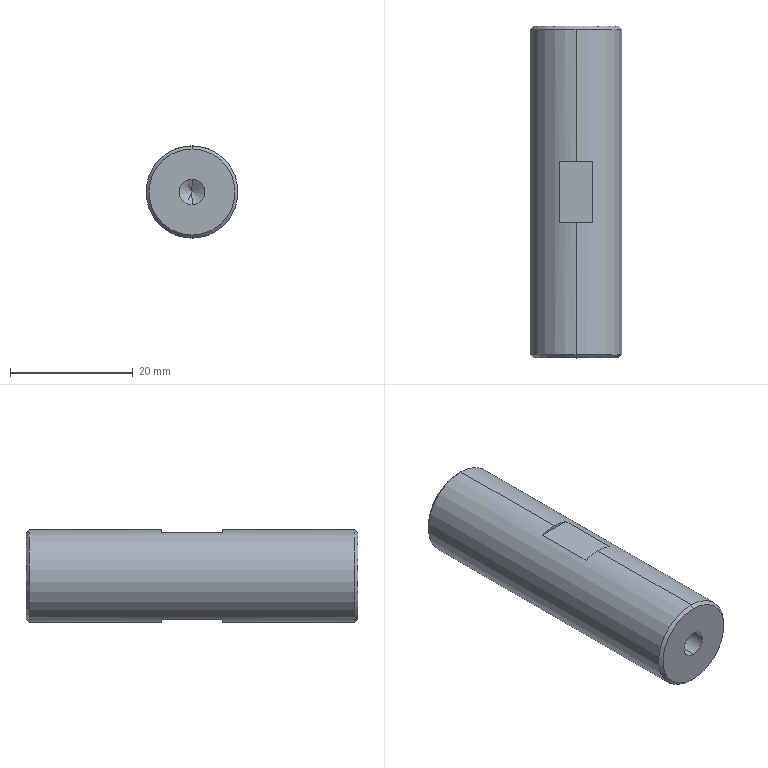Part | STEP file | ND25021-01-JDKM-17-TL | 1 solid | 22 faces | box 15 x 54 x 15 mm | volume 9140 mm3 | cone 8 | plane 8 | cylinder 6 | commonest cylinder face diameters 4.2 x4 15 x2
STEP:
#1=CARTESIAN_POINT('',(0.,0.,0.));
#2=DIRECTION('',(0.,0.,1.));
#3=DIRECTION('',(1.,0.,0.));
#4=AXIS2_PLACEMENT_3D('',#1,#2,#3);
#5=CARTESIAN_POINT('',(0.,-27.,-7.));
#6=VERTEX_POINT('',#5);
#7=CARTESIAN_POINT('',(0.,-27.,7.));
#8=VERTEX_POINT('',#7);
#9=CARTESIAN_POINT('',(0.,-27.,0.));
#10=DIRECTION('',(0.,-1.,0.));
#11=DIRECTION('',(0.,0.,1.));
#12=AXIS2_PLACEMENT_3D('',#9,#10,#11);
#13=CIRCLE('',#12,7.);
#14=CARTESIAN_POINT('',(0.,-26.5,0.));
#15=DIRECTION('',(0.,1.,0.));
#16=DIRECTION('',(0.,0.,1.));
#17=AXIS2_PLACEMENT_3D('',#14,#15,#16);
#18=CONICAL_SURFACE('',#17,7.5,0.7854);
#19=CARTESIAN_POINT('',(6.283,-0.5));
#20=DIRECTION('',(-1.,0.));
#21=VECTOR('',#20,1.);
#22=LINE('',#19,#21);
#23=(GEOMETRIC_REPRESENTATION_CONTEXT(2)PARAMETRIC_REPRESENTATION_CONTEXT()REPRESENTATION_CONTEXT('',''));
#24=DEFINITIONAL_REPRESENTATION('',(#22),#23);
#25=PCURVE('',#18,#24);
#26=CARTESIAN_POINT('',(0.,-27.,0.));
#27=DIRECTION('',(0.,1.,0.));
#28=DIRECTION('',(0.,0.,1.));
#29=AXIS2_PLACEMENT_3D('',#26,#27,#28);
#30=PLANE('',#29);
#31=CARTESIAN_POINT('',(7.,0.));
#32=CARTESIAN_POINT('',(7.,-12.124));
#33=CARTESIAN_POINT('',(-3.5,-6.062));
#34=CARTESIAN_POINT('',(-14.,0.));
#35=CARTESIAN_POINT('',(-3.5,6.062));
#36=CARTESIAN_POINT('',(7.,12.124));
#37=CARTESIAN_POINT('',(7.,0.));
#38=(BOUNDED_CURVE()B_SPLINE_CURVE(2,(#31,#32,#33,#34,#35,#36,#37),.UNSPECIFIED.,.T.,.F.)B_SPLINE_CURVE_WITH_KNOTS((1,2,2,2,2,1),(-2.094,0.,2.094,4.189,6.283,8.378),.UNSPECIFIED.)CURVE()GEOMETRIC_REPRESENTATION_ITEM()RATIONAL_B_SPLINE_CURVE((1.,0.5,1.,0.5,1.,0.5,1.))REPRESENTATION_ITEM(''));
#39=(GEOMETRIC_REPRESENTATION_CONTEXT(2)PARAMETRIC_REPRESENTATION_CONTEXT()REPRESENTATION_CONTEXT('',''));
#40=DEFINITIONAL_REPRESENTATION('',(#38),#39);
#41=PCURVE('',#30,#40);
#42=SURFACE_CURVE('',#13,(#25,#41),.PCURVE_S1.);
#43=EDGE_CURVE('',#6,#8,#42,.T.);
#44=ORIENTED_EDGE('',*,*,#43,.F.);
#45=CARTESIAN_POINT('',(0.,-26.5,-7.5));
#46=VERTEX_POINT('',#45);
#47=CARTESIAN_POINT('',(0.,-26.5,-7.5));
#48=DIRECTION('',(0.,0.7071,-0.7071));
#49=VECTOR('',#48,1.);
#50=LINE('',#47,#49);
#51=CARTESIAN_POINT('',(3.142,0.));
#52=DIRECTION('',(0.,1.));
#53=VECTOR('',#52,1.);
#54=LINE('',#51,#53);
#55=(GEOMETRIC_REPRESENTATION_CONTEXT(2)PARAMETRIC_REPRESENTATION_CONTEXT()REPRESENTATION_CONTEXT('',''));
#56=DEFINITIONAL_REPRESENTATION('',(#54),#55);
#57=PCURVE('',#18,#56);
#58=CARTESIAN_POINT('',(0.,-26.5,0.));
#59=DIRECTION('',(0.,1.,0.));
#60=DIRECTION('',(0.,0.,1.));
#61=AXIS2_PLACEMENT_3D('',#58,#59,#60);
#62=CONICAL_SURFACE('',#61,7.5,0.7854);
#63=CARTESIAN_POINT('',(3.142,0.));
#64=DIRECTION('',(0.,1.));
#65=VECTOR('',#64,1.);
#66=LINE('',#63,#65);
#67=(GEOMETRIC_REPRESENTATION_CONTEXT(2)PARAMETRIC_REPRESENTATION_CONTEXT()REPRESENTATION_CONTEXT('',''));
#68=DEFINITIONAL_REPRESENTATION('',(#66),#67);
#69=PCURVE('',#62,#68);
#70=SURFACE_CURVE('',#50,(#57,#69),.PCURVE_S1.);
#71=EDGE_CURVE('',#6,#46,#70,.T.);
#72=ORIENTED_EDGE('',*,*,#71,.T.);
#73=CARTESIAN_POINT('',(0.,-26.5,7.5));
#74=VERTEX_POINT('',#73);
#75=CARTESIAN_POINT('',(0.,-26.5,0.));
#76=DIRECTION('',(0.,1.,0.));
#77=DIRECTION('',(0.,0.,1.));
#78=AXIS2_PLACEMENT_3D('',#75,#76,#77);
#79=CIRCLE('',#78,7.5);
#80=CARTESIAN_POINT('',(0.,0.));
#81=DIRECTION('',(1.,0.));
#82=VECTOR('',#81,1.);
#83=LINE('',#80,#82);
#84=(GEOMETRIC_REPRESENTATION_CONTEXT(2)PARAMETRIC_REPRESENTATION_CONTEXT()REPRESENTATION_CONTEXT('',''));
#85=DEFINITIONAL_REPRESENTATION('',(#83),#84);
#86=PCURVE('',#18,#85);
#87=CARTESIAN_POINT('',(0.,27.,0.));
#88=DIRECTION('',(0.,-1.,0.));
#89=DIRECTION('',(0.,0.,-1.));
#90=AXIS2_PLACEMENT_3D('',#87,#88,#89);
#91=CYLINDRICAL_SURFACE('',#90,7.5);
#92=CARTESIAN_POINT('',(3.142,53.5));
#93=DIRECTION('',(-1.,0.));
#94=VECTOR('',#93,1.);
#95=LINE('',#92,#94);
#96=(GEOMETRIC_REPRESENTATION_CONTEXT(2)PARAMETRIC_REPRESENTATION_CONTEXT()REPRESENTATION_CONTEXT('',''));
#97=DEFINITIONAL_REPRESENTATION('',(#95),#96);
#98=PCURVE('',#91,#97);
#99=SURFACE_CURVE('',#79,(#86,#98),.PCURVE_S1.);
#100=EDGE_CURVE('',#74,#46,#99,.T.);
#101=ORIENTED_EDGE('',*,*,#100,.F.);
#102=CARTESIAN_POINT('',(0.,-26.5,7.5));
#103=DIRECTION('',(0.,0.7071,0.7071));
#104=VECTOR('',#103,1.);
#105=LINE('',#102,#104);
#106=CARTESIAN_POINT('',(0.,0.));
#107=DIRECTION('',(0.,1.));
#108=VECTOR('',#107,1.);
#109=LINE('',#106,#108);
#110=(GEOMETRIC_REPRESENTATION_CONTEXT(2)PARAMETRIC_REPRESENTATION_CONTEXT()REPRESENTATION_CONTEXT('',''));
#111=DEFINITIONAL_REPRESENTATION('',(#109),#110);
#112=PCURVE('',#18,#111);
#113=CARTESIAN_POINT('',(6.283,0.));
#114=DIRECTION('',(0.,1.));
#115=VECTOR('',#114,1.);
#116=LINE('',#113,#115);
#117=(GEOMETRIC_REPRESENTATION_CONTEXT(2)PARAMETRIC_REPRESENTATION_CONTEXT()REPRESENTATION_CONTEXT('',''));
#118=DEFINITIONAL_REPRESENTATION('',(#116),#117);
#119=PCURVE('',#62,#118);
#120=SURFACE_CURVE('',#105,(#112,#119),.PCURVE_S1.);
#121=EDGE_CURVE('',#8,#74,#120,.T.);
#122=ORIENTED_EDGE('',*,*,#121,.F.);
#123=EDGE_LOOP('',(#44,#72,#101,#122));
#124=FACE_BOUND('',#123,.T.);
#125=ADVANCED_FACE('',(#124),#18,.T.);
#126=CARTESIAN_POINT('',(0.,27.,7.));
#127=VERTEX_POINT('',#126);
#128=CARTESIAN_POINT('',(0.,27.,-7.));
#129=VERTEX_POINT('',#128);
#130=CARTESIAN_POINT('',(0.,27.,0.));
#131=DIRECTION('',(0.,1.,0.));
#132=DIRECTION('',(0.,0.,1.));
#133=AXIS2_PLACEMENT_3D('',#130,#131,#132);
#134=CIRCLE('',#133,7.);
#135=CARTESIAN_POINT('',(0.,27.,0.));
#136=DIRECTION('',(0.,-1.,0.));
#137=DIRECTION('',(0.,0.,-1.));
#138=AXIS2_PLACEMENT_3D('',#135,#136,#137);
#139=CONICAL_SURFACE('',#138,7.,0.7854);
#140=CARTESIAN_POINT('',(3.142,0.));
#141=DIRECTION('',(-1.,0.));
#142=VECTOR('',#141,1.);
#143=LINE('',#140,#142);
#144=(GEOMETRIC_REPRESENTATION_CONTEXT(2)PARAMETRIC_REPRESENTATION_CONTEXT()REPRESENTATION_CONTEXT('',''));
#145=DEFINITIONAL_REPRESENTATION('',(#143),#144);
#146=PCURVE('',#139,#145);
#147=CARTESIAN_POINT('',(0.,27.,0.));
#148=DIRECTION('',(0.,1.,0.));
#149=DIRECTION('',(0.,0.,1.));
#150=AXIS2_PLACEMENT_3D('',#147,#148,#149);
#151=PLANE('',#150);
#152=CARTESIAN_POINT('',(0.,0.));
#153=DIRECTION('',(1.,0.));
#154=AXIS2_PLACEMENT_2D('',#152,#153);
#155=CIRCLE('',#154,7.);
#156=(GEOMETRIC_REPRESENTATION_CONTEXT(2)PARAMETRIC_REPRESENTATION_CONTEXT()REPRESENTATION_CONTEXT('',''));
#157=DEFINITIONAL_REPRESENTATION('',(#155),#156);
#158=PCURVE('',#151,#157);
#159=SURFACE_CURVE('',#134,(#146,#158),.PCURVE_S1.);
#160=EDGE_CURVE('',#127,#129,#159,.T.);
#161=ORIENTED_EDGE('',*,*,#160,.F.);
#162=CARTESIAN_POINT('',(0.,26.5,7.5));
#163=VERTEX_POINT('',#162);
#164=CARTESIAN_POINT('',(0.,27.,7.));
#165=DIRECTION('',(0.,-0.7071,0.7071));
#166=VECTOR('',#165,1.);
#167=LINE('',#164,#166);
#168=CARTESIAN_POINT('',(3.142,0.));
#169=DIRECTION('',(0.,1.));
#170=VECTOR('',#169,1.);
#171=LINE('',#168,#170);
#172=(GEOMETRIC_REPRESENTATION_CONTEXT(2)PARAMETRIC_REPRESENTATION_CONTEXT()REPRESENTATION_CONTEXT('',''));
#173=DEFINITIONAL_REPRESENTATION('',(#171),#172);
#174=PCURVE('',#139,#173);
#175=CARTESIAN_POINT('',(0.,27.,0.));
#176=DIRECTION('',(0.,-1.,0.));
#177=DIRECTION('',(0.,0.,-1.));
#178=AXIS2_PLACEMENT_3D('',#175,#176,#177);
#179=CONICAL_SURFACE('',#178,7.,0.7854);
#180=CARTESIAN_POINT('',(3.142,0.));
#181=DIRECTION('',(0.,1.));
#182=VECTOR('',#181,1.);
#183=LINE('',#180,#182);
#184=(GEOMETRIC_REPRESENTATION_CONTEXT(2)PARAMETRIC_REPRESENTATION_CONTEXT()REPRESENTATION_CONTEXT('',''));
#185=DEFINITIONAL_REPRESENTATION('',(#183),#184);
#186=PCURVE('',#179,#185);
#187=SURFACE_CURVE('',#167,(#174,#186),.PCURVE_S1.);
#188=EDGE_CURVE('',#127,#163,#187,.T.);
#189=ORIENTED_EDGE('',*,*,#188,.T.);
#190=CARTESIAN_POINT('',(0.,26.5,-7.5));
#191=VERTEX_POINT('',#190);
#192=CARTESIAN_POINT('',(0.,26.5,0.));
#193=DIRECTION('',(0.,-1.,0.));
#194=DIRECTION('',(0.,0.,1.));
#195=AXIS2_PLACEMENT_3D('',#192,#193,#194);
#196=CIRCLE('',#195,7.5);
#197=CARTESIAN_POINT('',(-3.142,0.5));
#198=DIRECTION('',(1.,0.));
#199=VECTOR('',#198,1.);
#200=LINE('',#197,#199);
#201=(GEOMETRIC_REPRESENTATION_CONTEXT(2)PARAMETRIC_REPRESENTATION_CONTEXT()REPRESENTATION_CONTEXT('',''));
#202=DEFINITIONAL_REPRESENTATION('',(#200),#201);
#203=PCURVE('',#139,#202);
#204=CARTESIAN_POINT('',(-3.142,0.5));
#205=DIRECTION('',(1.,0.));
#206=VECTOR('',#205,1.);
#207=LINE('',#204,#206);
#208=(GEOMETRIC_REPRESENTATION_CONTEXT(2)PARAMETRIC_REPRESENTATION_CONTEXT()REPRESENTATION_CONTEXT('',''));
#209=DEFINITIONAL_REPRESENTATION('',(#207),#208);
#210=PCURVE('',#91,#209);
#211=SURFACE_CURVE('',#196,(#203,#210),.PCURVE_S1.);
#212=EDGE_CURVE('',#191,#163,#211,.T.);
#213=ORIENTED_EDGE('',*,*,#212,.F.);
#214=CARTESIAN_POINT('',(0.,27.,-7.));
#215=DIRECTION('',(0.,-0.7071,-0.7071));
#216=VECTOR('',#215,1.);
#217=LINE('',#214,#216);
#218=CARTESIAN_POINT('',(0.,0.));
#219=DIRECTION('',(0.,1.));
#220=VECTOR('',#219,1.);
#221=LINE('',#218,#220);
#222=(GEOMETRIC_REPRESENTATION_CONTEXT(2)PARAMETRIC_REPRESENTATION_CONTEXT()REPRESENTATION_CONTEXT('',''));
#223=DEFINITIONAL_REPRESENTATION('',(#221),#222);
#224=PCURVE('',#139,#223);
#225=CARTESIAN_POINT('',(6.283,0.));
#226=DIRECTION('',(0.,1.));
#227=VECTOR('',#226,1.);
#228=LINE('',#225,#227);
#229=(GEOMETRIC_REPRESENTATION_CONTEXT(2)PARAMETRIC_REPRESENTATION_CONTEXT()REPRESENTATION_CONTEXT('',''));
#230=DEFINITIONAL_REPRESENTATION('',(#228),#229);
#231=PCURVE('',#179,#230);
#232=SURFACE_CURVE('',#217,(#224,#231),.PCURVE_S1.);
#233=EDGE_CURVE('',#129,#191,#232,.T.);
#234=ORIENTED_EDGE('',*,*,#233,.F.);
#235=EDGE_LOOP('',(#161,#189,#213,#234));
#236=FACE_BOUND('',#235,.T.);
#237=ADVANCED_FACE('',(#236),#139,.T.);
#238=CARTESIAN_POINT('',(0.,14.6,2.1));
#239=VERTEX_POINT('',#238);
#240=CARTESIAN_POINT('',(0.,27.,2.1));
#241=VERTEX_POINT('',#240);
#242=CARTESIAN_POINT('',(0.,27.,2.1));
#243=DIRECTION('',(0.,1.,0.));
#244=VECTOR('',#243,1.);
#245=LINE('',#242,#244);
#246=CARTESIAN_POINT('',(0.,27.,0.));
#247=DIRECTION('',(0.,1.,0.));
#248=DIRECTION('',(0.,0.,1.));
#249=AXIS2_PLACEMENT_3D('',#246,#247,#248);
#250=CYLINDRICAL_SURFACE('',#249,2.1);
#251=CARTESIAN_POINT('',(6.283,0.));
#252=DIRECTION('',(0.,1.));
#253=VECTOR('',#252,1.);
#254=LINE('',#251,#253);
#255=(GEOMETRIC_REPRESENTATION_CONTEXT(2)PARAMETRIC_REPRESENTATION_CONTEXT()REPRESENTATION_CONTEXT('',''));
#256=DEFINITIONAL_REPRESENTATION('',(#254),#255);
#257=PCURVE('',#250,#256);
#258=CARTESIAN_POINT('',(0.,27.,0.));
#259=DIRECTION('',(0.,1.,0.));
#260=DIRECTION('',(0.,0.,1.));
#261=AXIS2_PLACEMENT_3D('',#258,#259,#260);
#262=CYLINDRICAL_SURFACE('',#261,2.1);
#263=CARTESIAN_POINT('',(0.,0.));
#264=DIRECTION('',(0.,1.));
#265=VECTOR('',#264,1.);
#266=LINE('',#263,#265);
#267=(GEOMETRIC_REPRESENTATION_CONTEXT(2)PARAMETRIC_REPRESENTATION_CONTEXT()REPRESENTATION_CONTEXT('',''));
#268=DEFINITIONAL_REPRESENTATION('',(#266),#267);
#269=PCURVE('',#262,#268);
#270=SURFACE_CURVE('',#245,(#257,#269),.PCURVE_S1.);
#271=EDGE_CURVE('',#239,#241,#270,.T.);
#272=ORIENTED_EDGE('',*,*,#271,.T.);
#273=CARTESIAN_POINT('',(0.,27.,-2.1));
#274=VERTEX_POINT('',#273);
#275=CARTESIAN_POINT('',(0.,27.,0.));
#276=DIRECTION('',(0.,1.,0.));
#277=DIRECTION('',(0.,0.,1.));
#278=AXIS2_PLACEMENT_3D('',#275,#276,#277);
#279=CIRCLE('',#278,2.1);
#280=CARTESIAN_POINT('',(0.,0.));
#281=DIRECTION('',(1.,0.));
#282=VECTOR('',#281,1.);
#283=LINE('',#280,#282);
#284=(GEOMETRIC_REPRESENTATION_CONTEXT(2)PARAMETRIC_REPRESENTATION_CONTEXT()REPRESENTATION_CONTEXT('',''));
#285=DEFINITIONAL_REPRESENTATION('',(#283),#284);
#286=PCURVE('',#250,#285);
#287=CARTESIAN_POINT('',(0.,0.));
#288=DIRECTION('',(1.,0.));
#289=AXIS2_PLACEMENT_2D('',#287,#288);
#290=CIRCLE('',#289,2.1);
#291=(GEOMETRIC_REPRESENTATION_CONTEXT(2)PARAMETRIC_REPRESENTATION_CONTEXT()REPRESENTATION_CONTEXT('',''));
#292=DEFINITIONAL_REPRESENTATION('',(#290),#291);
#293=PCURVE('',#151,#292);
#294=SURFACE_CURVE('',#279,(#286,#293),.PCURVE_S1.);
#295=EDGE_CURVE('',#274,#241,#294,.T.);
#296=ORIENTED_EDGE('',*,*,#295,.F.);
#297=CARTESIAN_POINT('',(0.,14.6,-2.1));
#298=VERTEX_POINT('',#297);
#299=CARTESIAN_POINT('',(0.,27.,-2.1));
#300=DIRECTION('',(0.,1.,0.));
#301=VECTOR('',#300,1.);
#302=LINE('',#299,#301);
#303=CARTESIAN_POINT('',(3.142,0.));
#304=DIRECTION('',(0.,1.));
#305=VECTOR('',#304,1.);
#306=LINE('',#303,#305);
#307=(GEOMETRIC_REPRESENTATION_CONTEXT(2)PARAMETRIC_REPRESENTATION_CONTEXT()REPRESENTATION_CONTEXT('',''));
#308=DEFINITIONAL_REPRESENTATION('',(#306),#307);
#309=PCURVE('',#250,#308);
#310=CARTESIAN_POINT('',(3.142,0.));
#311=DIRECTION('',(0.,1.));
#312=VECTOR('',#311,1.);
#313=LINE('',#310,#312);
#314=(GEOMETRIC_REPRESENTATION_CONTEXT(2)PARAMETRIC_REPRESENTATION_CONTEXT()REPRESENTATION_CONTEXT('',''));
#315=DEFINITIONAL_REPRESENTATION('',(#313),#314);
#316=PCURVE('',#262,#315);
#317=SURFACE_CURVE('',#302,(#309,#316),.PCURVE_S1.);
#318=EDGE_CURVE('',#298,#274,#317,.T.);
#319=ORIENTED_EDGE('',*,*,#318,.F.);
#320=CARTESIAN_POINT('',(0.,14.6,0.));
#321=DIRECTION('',(0.,1.,0.));
#322=DIRECTION('',(0.,0.,1.));
#323=AXIS2_PLACEMENT_3D('',#320,#321,#322);
#324=CIRCLE('',#323,2.1);
#325=CARTESIAN_POINT('',(0.,-12.4));
#326=DIRECTION('',(1.,0.));
#327=VECTOR('',#326,1.);
#328=LINE('',#325,#327);
#329=(GEOMETRIC_REPRESENTATION_CONTEXT(2)PARAMETRIC_REPRESENTATION_CONTEXT()REPRESENTATION_CONTEXT('',''));
#330=DEFINITIONAL_REPRESENTATION('',(#328),#329);
#331=PCURVE('',#250,#330);
#332=CARTESIAN_POINT('',(0.,14.6,0.));
#333=DIRECTION('',(0.,1.,0.));
#334=DIRECTION('',(0.,0.,1.));
#335=AXIS2_PLACEMENT_3D('',#332,#333,#334);
#336=CONICAL_SURFACE('',#335,2.1,1.03);
#337=CARTESIAN_POINT('',(0.,0.));
#338=DIRECTION('',(1.,0.));
#339=VECTOR('',#338,1.);
#340=LINE('',#337,#339);
#341=(GEOMETRIC_REPRESENTATION_CONTEXT(2)PARAMETRIC_REPRESENTATION_CONTEXT()REPRESENTATION_CONTEXT('',''));
#342=DEFINITIONAL_REPRESENTATION('',(#340),#341);
#343=PCURVE('',#336,#342);
#344=SURFACE_CURVE('',#324,(#331,#343),.PCURVE_S1.);
#345=EDGE_CURVE('',#298,#239,#344,.T.);
#346=ORIENTED_EDGE('',*,*,#345,.T.);
#347=EDGE_LOOP('',(#272,#296,#319,#346));
#348=FACE_BOUND('',#347,.F.);
#349=ADVANCED_FACE('',(#348),#250,.F.);
#350=ORIENTED_EDGE('',*,*,#345,.F.);
#351=CARTESIAN_POINT('',(0.,13.338,0.));
#352=VERTEX_POINT('',#351);
#353=CARTESIAN_POINT('',(0.,14.6,-2.1));
#354=DIRECTION('',(0.,0.515,-0.8572));
#355=VECTOR('',#354,1.);
#356=LINE('',#353,#355);
#357=CARTESIAN_POINT('',(3.142,0.));
#358=DIRECTION('',(0.,1.));
#359=VECTOR('',#358,1.);
#360=LINE('',#357,#359);
#361=(GEOMETRIC_REPRESENTATION_CONTEXT(2)PARAMETRIC_REPRESENTATION_CONTEXT()REPRESENTATION_CONTEXT('',''));
#362=DEFINITIONAL_REPRESENTATION('',(#360),#361);
#363=PCURVE('',#336,#362);
#364=CARTESIAN_POINT('',(0.,14.6,0.));
#365=DIRECTION('',(0.,1.,0.));
#366=DIRECTION('',(0.,0.,1.));
#367=AXIS2_PLACEMENT_3D('',#364,#365,#366);
#368=CONICAL_SURFACE('',#367,2.1,1.03);
#369=CARTESIAN_POINT('',(3.142,0.));
#370=DIRECTION('',(0.,1.));
#371=VECTOR('',#370,1.);
#372=LINE('',#369,#371);
#373=(GEOMETRIC_REPRESENTATION_CONTEXT(2)PARAMETRIC_REPRESENTATION_CONTEXT()REPRESENTATION_CONTEXT('',''));
#374=DEFINITIONAL_REPRESENTATION('',(#372),#373);
#375=PCURVE('',#368,#374);
#376=SURFACE_CURVE('',#356,(#363,#375),.PCURVE_S1.);
#377=EDGE_CURVE('',#352,#298,#376,.T.);
#378=ORIENTED_EDGE('',*,*,#377,.F.);
#379=CARTESIAN_POINT('',(0.,14.6,2.1));
#380=DIRECTION('',(0.,0.515,0.8572));
#381=VECTOR('',#380,1.);
#382=LINE('',#379,#381);
#383=CARTESIAN_POINT('',(6.283,0.));
#384=DIRECTION('',(0.,1.));
#385=VECTOR('',#384,1.);
#386=LINE('',#383,#385);
#387=(GEOMETRIC_REPRESENTATION_CONTEXT(2)PARAMETRIC_REPRESENTATION_CONTEXT()REPRESENTATION_CONTEXT('',''));
#388=DEFINITIONAL_REPRESENTATION('',(#386),#387);
#389=PCURVE('',#336,#388);
#390=CARTESIAN_POINT('',(0.,0.));
#391=DIRECTION('',(0.,1.));
#392=VECTOR('',#391,1.);
#393=LINE('',#390,#392);
#394=(GEOMETRIC_REPRESENTATION_CONTEXT(2)PARAMETRIC_REPRESENTATION_CONTEXT()REPRESENTATION_CONTEXT('',''));
#395=DEFINITIONAL_REPRESENTATION('',(#393),#394);
#396=PCURVE('',#368,#395);
#397=SURFACE_CURVE('',#382,(#389,#396),.PCURVE_S1.);
#398=EDGE_CURVE('',#352,#239,#397,.T.);
#399=ORIENTED_EDGE('',*,*,#398,.T.);
#400=EDGE_LOOP('',(#350,#378,#399));
#401=FACE_BOUND('',#400,.F.);
#402=ADVANCED_FACE('',(#401),#336,.F.);
#403=CARTESIAN_POINT('',(0.,-14.6,-2.1));
#404=VERTEX_POINT('',#403);
#405=CARTESIAN_POINT('',(0.,-27.,-2.1));
#406=VERTEX_POINT('',#405);
#407=CARTESIAN_POINT('',(0.,-27.,-2.1));
#408=DIRECTION('',(0.,-1.,0.));
#409=VECTOR('',#408,1.);
#410=LINE('',#407,#409);
#411=CARTESIAN_POINT('',(0.,-27.,0.));
#412=DIRECTION('',(0.,-1.,0.));
#413=DIRECTION('',(0.,0.,-1.));
#414=AXIS2_PLACEMENT_3D('',#411,#412,#413);
#415=CYLINDRICAL_SURFACE('',#414,2.1);
#416=CARTESIAN_POINT('',(6.283,0.));
#417=DIRECTION('',(0.,1.));
#418=VECTOR('',#417,1.);
#419=LINE('',#416,#418);
#420=(GEOMETRIC_REPRESENTATION_CONTEXT(2)PARAMETRIC_REPRESENTATION_CONTEXT()REPRESENTATION_CONTEXT('',''));
#421=DEFINITIONAL_REPRESENTATION('',(#419),#420);
#422=PCURVE('',#415,#421);
#423=CARTESIAN_POINT('',(0.,-27.,0.));
#424=DIRECTION('',(0.,-1.,0.));
#425=DIRECTION('',(0.,0.,-1.));
#426=AXIS2_PLACEMENT_3D('',#423,#424,#425);
#427=CYLINDRICAL_SURFACE('',#426,2.1);
#428=CARTESIAN_POINT('',(0.,0.));
#429=DIRECTION('',(0.,1.));
#430=VECTOR('',#429,1.);
#431=LINE('',#428,#430);
#432=(GEOMETRIC_REPRESENTATION_CONTEXT(2)PARAMETRIC_REPRESENTATION_CONTEXT()REPRESENTATION_CONTEXT('',''));
#433=DEFINITIONAL_REPRESENTATION('',(#431),#432);
#434=PCURVE('',#427,#433);
#435=SURFACE_CURVE('',#410,(#422,#434),.PCURVE_S1.);
#436=EDGE_CURVE('',#404,#406,#435,.T.);
#437=ORIENTED_EDGE('',*,*,#436,.T.);
#438=CARTESIAN_POINT('',(0.,-27.,2.1));
#439=VERTEX_POINT('',#438);
#440=CARTESIAN_POINT('',(0.,-27.,0.));
#441=DIRECTION('',(0.,-1.,0.));
#442=DIRECTION('',(0.,0.,-1.));
#443=AXIS2_PLACEMENT_3D('',#440,#441,#442);
#444=CIRCLE('',#443,2.1);
#445=CARTESIAN_POINT('',(0.,0.));
#446=DIRECTION('',(1.,0.));
#447=VECTOR('',#446,1.);
#448=LINE('',#445,#447);
#449=(GEOMETRIC_REPRESENTATION_CONTEXT(2)PARAMETRIC_REPRESENTATION_CONTEXT()REPRESENTATION_CONTEXT('',''));
#450=DEFINITIONAL_REPRESENTATION('',(#448),#449);
#451=PCURVE('',#415,#450);
#452=CARTESIAN_POINT('',(-2.1,0.));
#453=CARTESIAN_POINT('',(-2.1,3.637));
#454=CARTESIAN_POINT('',(1.05,1.819));
#455=CARTESIAN_POINT('',(4.2,0.));
#456=CARTESIAN_POINT('',(1.05,-1.819));
#457=CARTESIAN_POINT('',(-2.1,-3.637));
#458=CARTESIAN_POINT('',(-2.1,0.));
#459=(BOUNDED_CURVE()B_SPLINE_CURVE(2,(#452,#453,#454,#455,#456,#457,#458),.UNSPECIFIED.,.T.,.F.)B_SPLINE_CURVE_WITH_KNOTS((1,2,2,2,2,1),(-2.094,0.,2.094,4.189,6.283,8.378),.UNSPECIFIED.)CURVE()GEOMETRIC_REPRESENTATION_ITEM()RATIONAL_B_SPLINE_CURVE((1.,0.5,1.,0.5,1.,0.5,1.))REPRESENTATION_ITEM(''));
#460=(GEOMETRIC_REPRESENTATION_CONTEXT(2)PARAMETRIC_REPRESENTATION_CONTEXT()REPRESENTATION_CONTEXT('',''));
#461=DEFINITIONAL_REPRESENTATION('',(#459),#460);
#462=PCURVE('',#30,#461);
#463=SURFACE_CURVE('',#444,(#451,#462),.PCURVE_S1.);
#464=EDGE_CURVE('',#439,#406,#463,.T.);
#465=ORIENTED_EDGE('',*,*,#464,.F.);
#466=CARTESIAN_POINT('',(0.,-14.6,2.1));
#467=VERTEX_POINT('',#466);
#468=CARTESIAN_POINT('',(0.,-27.,2.1));
#469=DIRECTION('',(0.,-1.,0.));
#470=VECTOR('',#469,1.);
#471=LINE('',#468,#470);
#472=CARTESIAN_POINT('',(3.142,0.));
#473=DIRECTION('',(0.,1.));
#474=VECTOR('',#473,1.);
#475=LINE('',#472,#474);
#476=(GEOMETRIC_REPRESENTATION_CONTEXT(2)PARAMETRIC_REPRESENTATION_CONTEXT()REPRESENTATION_CONTEXT('',''));
#477=DEFINITIONAL_REPRESENTATION('',(#475),#476);
#478=PCURVE('',#415,#477);
#479=CARTESIAN_POINT('',(3.142,0.));
#480=DIRECTION('',(0.,1.));
#481=VECTOR('',#480,1.);
#482=LINE('',#479,#481);
#483=(GEOMETRIC_REPRESENTATION_CONTEXT(2)PARAMETRIC_REPRESENTATION_CONTEXT()REPRESENTATION_CONTEXT('',''));
#484=DEFINITIONAL_REPRESENTATION('',(#482),#483);
#485=PCURVE('',#427,#484);
#486=SURFACE_CURVE('',#471,(#478,#485),.PCURVE_S1.);
#487=EDGE_CURVE('',#467,#439,#486,.T.);
#488=ORIENTED_EDGE('',*,*,#487,.F.);
#489=CARTESIAN_POINT('',(0.,-14.6,0.));
#490=DIRECTION('',(0.,-1.,0.));
#491=DIRECTION('',(0.,0.,-1.));
#492=AXIS2_PLACEMENT_3D('',#489,#490,#491);
#493=CIRCLE('',#492,2.1);
#494=CARTESIAN_POINT('',(0.,-12.4));
#495=DIRECTION('',(1.,0.));
#496=VECTOR('',#495,1.);
#497=LINE('',#494,#496);
#498=(GEOMETRIC_REPRESENTATION_CONTEXT(2)PARAMETRIC_REPRESENTATION_CONTEXT()REPRESENTATION_CONTEXT('',''));
#499=DEFINITIONAL_REPRESENTATION('',(#497),#498);
#500=PCURVE('',#415,#499);
#501=CARTESIAN_POINT('',(0.,-14.6,0.));
#502=DIRECTION('',(0.,-1.,0.));
#503=DIRECTION('',(0.,0.,-1.));
#504=AXIS2_PLACEMENT_3D('',#501,#502,#503);
#505=CONICAL_SURFACE('',#504,2.1,1.03);
#506=CARTESIAN_POINT('',(0.,0.));
#507=DIRECTION('',(1.,0.));
#508=VECTOR('',#507,1.);
#509=LINE('',#506,#508);
#510=(GEOMETRIC_REPRESENTATION_CONTEXT(2)PARAMETRIC_REPRESENTATION_CONTEXT()REPRESENTATION_CONTEXT('',''));
#511=DEFINITIONAL_REPRESENTATION('',(#509),#510);
#512=PCURVE('',#505,#511);
#513=SURFACE_CURVE('',#493,(#500,#512),.PCURVE_S1.);
#514=EDGE_CURVE('',#467,#404,#513,.T.);
#515=ORIENTED_EDGE('',*,*,#514,.T.);
#516=EDGE_LOOP('',(#437,#465,#488,#515));
#517=FACE_BOUND('',#516,.F.);
#518=ADVANCED_FACE('',(#517),#415,.F.);
#519=ORIENTED_EDGE('',*,*,#514,.F.);
#520=CARTESIAN_POINT('',(0.,-13.338,0.));
#521=VERTEX_POINT('',#520);
#522=CARTESIAN_POINT('',(0.,-14.6,2.1));
#523=DIRECTION('',(0.,-0.515,0.8572));
#524=VECTOR('',#523,1.);
#525=LINE('',#522,#524);
#526=CARTESIAN_POINT('',(3.142,0.));
#527=DIRECTION('',(0.,1.));
#528=VECTOR('',#527,1.);
#529=LINE('',#526,#528);
#530=(GEOMETRIC_REPRESENTATION_CONTEXT(2)PARAMETRIC_REPRESENTATION_CONTEXT()REPRESENTATION_CONTEXT('',''));
#531=DEFINITIONAL_REPRESENTATION('',(#529),#530);
#532=PCURVE('',#505,#531);
#533=CARTESIAN_POINT('',(0.,-14.6,0.));
#534=DIRECTION('',(0.,-1.,0.));
#535=DIRECTION('',(0.,0.,-1.));
#536=AXIS2_PLACEMENT_3D('',#533,#534,#535);
#537=CONICAL_SURFACE('',#536,2.1,1.03);
#538=CARTESIAN_POINT('',(3.142,0.));
#539=DIRECTION('',(0.,1.));
#540=VECTOR('',#539,1.);
#541=LINE('',#538,#540);
#542=(GEOMETRIC_REPRESENTATION_CONTEXT(2)PARAMETRIC_REPRESENTATION_CONTEXT()REPRESENTATION_CONTEXT('',''));
#543=DEFINITIONAL_REPRESENTATION('',(#541),#542);
#544=PCURVE('',#537,#543);
#545=SURFACE_CURVE('',#525,(#532,#544),.PCURVE_S1.);
#546=EDGE_CURVE('',#521,#467,#545,.T.);
#547=ORIENTED_EDGE('',*,*,#546,.F.);
#548=CARTESIAN_POINT('',(0.,-14.6,-2.1));
#549=DIRECTION('',(0.,-0.515,-0.8572));
#550=VECTOR('',#549,1.);
#551=LINE('',#548,#550);
#552=CARTESIAN_POINT('',(6.283,0.));
#553=DIRECTION('',(0.,1.));
#554=VECTOR('',#553,1.);
#555=LINE('',#552,#554);
#556=(GEOMETRIC_REPRESENTATION_CONTEXT(2)PARAMETRIC_REPRESENTATION_CONTEXT()REPRESENTATION_CONTEXT('',''));
#557=DEFINITIONAL_REPRESENTATION('',(#555),#556);
#558=PCURVE('',#505,#557);
#559=CARTESIAN_POINT('',(0.,0.));
#560=DIRECTION('',(0.,1.));
#561=VECTOR('',#560,1.);
#562=LINE('',#559,#561);
#563=(GEOMETRIC_REPRESENTATION_CONTEXT(2)PARAMETRIC_REPRESENTATION_CONTEXT()REPRESENTATION_CONTEXT('',''));
#564=DEFINITIONAL_REPRESENTATION('',(#562),#563);
#565=PCURVE('',#537,#564);
#566=SURFACE_CURVE('',#551,(#558,#565),.PCURVE_S1.);
#567=EDGE_CURVE('',#521,#404,#566,.T.);
#568=ORIENTED_EDGE('',*,*,#567,.T.);
#569=EDGE_LOOP('',(#519,#547,#568));
#570=FACE_BOUND('',#569,.F.);
#571=ADVANCED_FACE('',(#570),#505,.F.);
#572=ORIENTED_EDGE('',*,*,#212,.T.);
#573=CARTESIAN_POINT('',(0.,5.,7.5));
#574=VERTEX_POINT('',#573);
#575=CARTESIAN_POINT('',(0.,27.,7.5));
#576=DIRECTION('',(0.,-1.,0.));
#577=VECTOR('',#576,1.);
#578=LINE('',#575,#577);
#579=CARTESIAN_POINT('',(3.142,0.));
#580=DIRECTION('',(0.,1.));
#581=VECTOR('',#580,1.);
#582=LINE('',#579,#581);
#583=(GEOMETRIC_REPRESENTATION_CONTEXT(2)PARAMETRIC_REPRESENTATION_CONTEXT()REPRESENTATION_CONTEXT('',''));
#584=DEFINITIONAL_REPRESENTATION('',(#582),#583);
#585=PCURVE('',#91,#584);
#586=CARTESIAN_POINT('',(0.,27.,0.));
#587=DIRECTION('',(0.,-1.,0.));
#588=DIRECTION('',(0.,0.,-1.));
#589=AXIS2_PLACEMENT_3D('',#586,#587,#588);
#590=CYLINDRICAL_SURFACE('',#589,7.5);
#591=CARTESIAN_POINT('',(3.142,0.));
#592=DIRECTION('',(0.,1.));
#593=VECTOR('',#592,1.);
#594=LINE('',#591,#593);
#595=(GEOMETRIC_REPRESENTATION_CONTEXT(2)PARAMETRIC_REPRESENTATION_CONTEXT()REPRESENTATION_CONTEXT('',''));
#596=DEFINITIONAL_REPRESENTATION('',(#594),#595);
#597=PCURVE('',#590,#596);
#598=SURFACE_CURVE('',#578,(#585,#597),.PCURVE_S1.);
#599=EDGE_CURVE('',#163,#574,#598,.T.);
#600=ORIENTED_EDGE('',*,*,#599,.T.);
#601=CARTESIAN_POINT('',(2.693,5.,7.));
#602=VERTEX_POINT('',#601);
#603=CARTESIAN_POINT('',(0.,5.,0.));
#604=DIRECTION('',(0.,1.,0.));
#605=DIRECTION('',(0.,0.,1.));
#606=AXIS2_PLACEMENT_3D('',#603,#604,#605);
#607=CIRCLE('',#606,7.5);
#608=CARTESIAN_POINT('',(3.142,22.));
#609=DIRECTION('',(-1.,0.));
#610=VECTOR('',#609,1.);
#611=LINE('',#608,#610);
#612=(GEOMETRIC_REPRESENTATION_CONTEXT(2)PARAMETRIC_REPRESENTATION_CONTEXT()REPRESENTATION_CONTEXT('',''));
#613=DEFINITIONAL_REPRESENTATION('',(#611),#612);
#614=PCURVE('',#91,#613);
#615=CARTESIAN_POINT('',(0.,5.,0.));
#616=DIRECTION('',(0.,1.,0.));
#617=DIRECTION('',(0.,0.,1.));
#618=AXIS2_PLACEMENT_3D('',#615,#616,#617);
#619=PLANE('',#618);
#620=CARTESIAN_POINT('',(0.,0.));
#621=DIRECTION('',(1.,0.));
#622=AXIS2_PLACEMENT_2D('',#620,#621);
#623=CIRCLE('',#622,7.5);
#624=(GEOMETRIC_REPRESENTATION_CONTEXT(2)PARAMETRIC_REPRESENTATION_CONTEXT()REPRESENTATION_CONTEXT('',''));
#625=DEFINITIONAL_REPRESENTATION('',(#623),#624);
#626=PCURVE('',#619,#625);
#627=SURFACE_CURVE('',#607,(#614,#626),.PCURVE_S1.);
#628=EDGE_CURVE('',#574,#602,#627,.T.);
#629=ORIENTED_EDGE('',*,*,#628,.T.);
#630=CARTESIAN_POINT('',(2.693,-5.,7.));
#631=VERTEX_POINT('',#630);
#632=CARTESIAN_POINT('',(2.693,-5.,7.));
#633=DIRECTION('',(0.,1.,0.));
#634=VECTOR('',#633,1.);
#635=LINE('',#632,#634);
#636=CARTESIAN_POINT('',(2.774,32.));
#637=DIRECTION('',(0.,-1.));
#638=VECTOR('',#637,1.);
#639=LINE('',#636,#638);
#640=(GEOMETRIC_REPRESENTATION_CONTEXT(2)PARAMETRIC_REPRESENTATION_CONTEXT()REPRESENTATION_CONTEXT('',''));
#641=DEFINITIONAL_REPRESENTATION('',(#639),#640);
#642=PCURVE('',#91,#641);
#643=CARTESIAN_POINT('',(-2.693,-5.,7.));
#644=DIRECTION('',(0.,0.,-1.));
#645=DIRECTION('',(-1.,0.,0.));
#646=AXIS2_PLACEMENT_3D('',#643,#644,#645);
#647=PLANE('',#646);
#648=CARTESIAN_POINT('',(-5.385,0.));
#649=DIRECTION('',(0.,1.));
#650=VECTOR('',#649,1.);
#651=LINE('',#648,#650);
#652=(GEOMETRIC_REPRESENTATION_CONTEXT(2)PARAMETRIC_REPRESENTATION_CONTEXT()REPRESENTATION_CONTEXT('',''));
#653=DEFINITIONAL_REPRESENTATION('',(#651),#652);
#654=PCURVE('',#647,#653);
#655=SURFACE_CURVE('',#635,(#642,#654),.PCURVE_S1.);
#656=EDGE_CURVE('',#631,#602,#655,.T.);
#657=ORIENTED_EDGE('',*,*,#656,.F.);
#658=CARTESIAN_POINT('',(0.,-5.,7.5));
#659=VERTEX_POINT('',#658);
#660=CARTESIAN_POINT('',(0.,-5.,0.));
#661=DIRECTION('',(0.,1.,0.));
#662=DIRECTION('',(0.,0.,1.));
#663=AXIS2_PLACEMENT_3D('',#660,#661,#662);
#664=CIRCLE('',#663,7.5);
#665=CARTESIAN_POINT('',(3.142,32.));
#666=DIRECTION('',(-1.,0.));
#667=VECTOR('',#666,1.);
#668=LINE('',#665,#667);
#669=(GEOMETRIC_REPRESENTATION_CONTEXT(2)PARAMETRIC_REPRESENTATION_CONTEXT()REPRESENTATION_CONTEXT('',''));
#670=DEFINITIONAL_REPRESENTATION('',(#668),#669);
#671=PCURVE('',#91,#670);
#672=CARTESIAN_POINT('',(0.,-5.,0.));
#673=DIRECTION('',(0.,1.,0.));
#674=DIRECTION('',(0.,0.,1.));
#675=AXIS2_PLACEMENT_3D('',#672,#673,#674);
#676=PLANE('',#675);
#677=CARTESIAN_POINT('',(0.,0.));
#678=DIRECTION('',(1.,0.));
#679=AXIS2_PLACEMENT_2D('',#677,#678);
#680=CIRCLE('',#679,7.5);
#681=(GEOMETRIC_REPRESENTATION_CONTEXT(2)PARAMETRIC_REPRESENTATION_CONTEXT()REPRESENTATION_CONTEXT('',''));
#682=DEFINITIONAL_REPRESENTATION('',(#680),#681);
#683=PCURVE('',#676,#682);
#684=SURFACE_CURVE('',#664,(#671,#683),.PCURVE_S1.);
#685=EDGE_CURVE('',#659,#631,#684,.T.);
#686=ORIENTED_EDGE('',*,*,#685,.F.);
#687=CARTESIAN_POINT('',(0.,27.,7.5));
#688=DIRECTION('',(0.,-1.,0.));
#689=VECTOR('',#688,1.);
#690=LINE('',#687,#689);
#691=CARTESIAN_POINT('',(3.142,0.));
#692=DIRECTION('',(0.,1.));
#693=VECTOR('',#692,1.);
#694=LINE('',#691,#693);
#695=(GEOMETRIC_REPRESENTATION_CONTEXT(2)PARAMETRIC_REPRESENTATION_CONTEXT()REPRESENTATION_CONTEXT('',''));
#696=DEFINITIONAL_REPRESENTATION('',(#694),#695);
#697=PCURVE('',#91,#696);
#698=CARTESIAN_POINT('',(3.142,0.));
#699=DIRECTION('',(0.,1.));
#700=VECTOR('',#699,1.);
#701=LINE('',#698,#700);
#702=(GEOMETRIC_REPRESENTATION_CONTEXT(2)PARAMETRIC_REPRESENTATION_CONTEXT()REPRESENTATION_CONTEXT('',''));
#703=DEFINITIONAL_REPRESENTATION('',(#701),#702);
#704=PCURVE('',#590,#703);
#705=SURFACE_CURVE('',#690,(#697,#704),.PCURVE_S1.);
#706=EDGE_CURVE('',#659,#74,#705,.T.);
#707=ORIENTED_EDGE('',*,*,#706,.T.);
#708=ORIENTED_EDGE('',*,*,#100,.T.);
#709=CARTESIAN_POINT('',(0.,-5.,-7.5));
#710=VERTEX_POINT('',#709);
#711=CARTESIAN_POINT('',(0.,27.,-7.5));
#712=DIRECTION('',(0.,-1.,0.));
#713=VECTOR('',#712,1.);
#714=LINE('',#711,#713);
#715=CARTESIAN_POINT('',(0.,0.));
#716=DIRECTION('',(0.,1.));
#717=VECTOR('',#716,1.);
#718=LINE('',#715,#717);
#719=(GEOMETRIC_REPRESENTATION_CONTEXT(2)PARAMETRIC_REPRESENTATION_CONTEXT()REPRESENTATION_CONTEXT('',''));
#720=DEFINITIONAL_REPRESENTATION('',(#718),#719);
#721=PCURVE('',#91,#720);
#722=CARTESIAN_POINT('',(6.283,0.));
#723=DIRECTION('',(0.,1.));
#724=VECTOR('',#723,1.);
#725=LINE('',#722,#724);
#726=(GEOMETRIC_REPRESENTATION_CONTEXT(2)PARAMETRIC_REPRESENTATION_CONTEXT()REPRESENTATION_CONTEXT('',''));
#727=DEFINITIONAL_REPRESENTATION('',(#725),#726);
#728=PCURVE('',#590,#727);
#729=SURFACE_CURVE('',#714,(#721,#728),.PCURVE_S1.);
#730=EDGE_CURVE('',#710,#46,#729,.T.);
#731=ORIENTED_EDGE('',*,*,#730,.F.);
#732=CARTESIAN_POINT('',(2.693,-5.,-7.));
#733=VERTEX_POINT('',#732);
#734=CARTESIAN_POINT('',(0.,-5.,0.));
#735=DIRECTION('',(0.,1.,0.));
#736=DIRECTION('',(0.,0.,1.));
#737=AXIS2_PLACEMENT_3D('',#734,#735,#736);
#738=CIRCLE('',#737,7.5);
#739=CARTESIAN_POINT('',(3.142,32.));
#740=DIRECTION('',(-1.,0.));
#741=VECTOR('',#740,1.);
#742=LINE('',#739,#741);
#743=(GEOMETRIC_REPRESENTATION_CONTEXT(2)PARAMETRIC_REPRESENTATION_CONTEXT()REPRESENTATION_CONTEXT('',''));
#744=DEFINITIONAL_REPRESENTATION('',(#742),#743);
#745=PCURVE('',#91,#744);
#746=CARTESIAN_POINT('',(0.,-5.,0.));
#747=DIRECTION('',(0.,1.,0.));
#748=DIRECTION('',(0.,0.,1.));
#749=AXIS2_PLACEMENT_3D('',#746,#747,#748);
#750=PLANE('',#749);
#751=CARTESIAN_POINT('',(0.,0.));
#752=DIRECTION('',(1.,0.));
#753=AXIS2_PLACEMENT_2D('',#751,#752);
#754=CIRCLE('',#753,7.5);
#755=(GEOMETRIC_REPRESENTATION_CONTEXT(2)PARAMETRIC_REPRESENTATION_CONTEXT()REPRESENTATION_CONTEXT('',''));
#756=DEFINITIONAL_REPRESENTATION('',(#754),#755);
#757=PCURVE('',#750,#756);
#758=SURFACE_CURVE('',#738,(#745,#757),.PCURVE_S1.);
#759=EDGE_CURVE('',#733,#710,#758,.T.);
#760=ORIENTED_EDGE('',*,*,#759,.F.);
#761=CARTESIAN_POINT('',(2.693,5.,-7.));
#762=VERTEX_POINT('',#761);
#763=CARTESIAN_POINT('',(2.693,-5.,-7.));
#764=DIRECTION('',(0.,1.,0.));
#765=VECTOR('',#764,1.);
#766=LINE('',#763,#765);
#767=CARTESIAN_POINT('',(0.3672,32.));
#768=DIRECTION('',(0.,-1.));
#769=VECTOR('',#768,1.);
#770=LINE('',#767,#769);
#771=(GEOMETRIC_REPRESENTATION_CONTEXT(2)PARAMETRIC_REPRESENTATION_CONTEXT()REPRESENTATION_CONTEXT('',''));
#772=DEFINITIONAL_REPRESENTATION('',(#770),#771);
#773=PCURVE('',#91,#772);
#774=CARTESIAN_POINT('',(-2.693,-5.,-7.));
#775=DIRECTION('',(0.,0.,1.));
#776=DIRECTION('',(1.,0.,0.));
#777=AXIS2_PLACEMENT_3D('',#774,#775,#776);
#778=PLANE('',#777);
#779=CARTESIAN_POINT('',(5.385,0.));
#780=DIRECTION('',(0.,1.));
#781=VECTOR('',#780,1.);
#782=LINE('',#779,#781);
#783=(GEOMETRIC_REPRESENTATION_CONTEXT(2)PARAMETRIC_REPRESENTATION_CONTEXT()REPRESENTATION_CONTEXT('',''));
#784=DEFINITIONAL_REPRESENTATION('',(#782),#783);
#785=PCURVE('',#778,#784);
#786=SURFACE_CURVE('',#766,(#773,#785),.PCURVE_S1.);
#787=EDGE_CURVE('',#733,#762,#786,.T.);
#788=ORIENTED_EDGE('',*,*,#787,.T.);
#789=CARTESIAN_POINT('',(0.,5.,-7.5));
#790=VERTEX_POINT('',#789);
#791=CARTESIAN_POINT('',(0.,5.,0.));
#792=DIRECTION('',(0.,1.,0.));
#793=DIRECTION('',(0.,0.,1.));
#794=AXIS2_PLACEMENT_3D('',#791,#792,#793);
#795=CIRCLE('',#794,7.5);
#796=CARTESIAN_POINT('',(3.142,22.));
#797=DIRECTION('',(-1.,0.));
#798=VECTOR('',#797,1.);
#799=LINE('',#796,#798);
#800=(GEOMETRIC_REPRESENTATION_CONTEXT(2)PARAMETRIC_REPRESENTATION_CONTEXT()REPRESENTATION_CONTEXT('',''));
#801=DEFINITIONAL_REPRESENTATION('',(#799),#800);
#802=PCURVE('',#91,#801);
#803=CARTESIAN_POINT('',(0.,5.,0.));
#804=DIRECTION('',(0.,1.,0.));
#805=DIRECTION('',(0.,0.,1.));
#806=AXIS2_PLACEMENT_3D('',#803,#804,#805);
#807=PLANE('',#806);
#808=CARTESIAN_POINT('',(0.,0.));
#809=DIRECTION('',(1.,0.));
#810=AXIS2_PLACEMENT_2D('',#808,#809);
#811=CIRCLE('',#810,7.5);
#812=(GEOMETRIC_REPRESENTATION_CONTEXT(2)PARAMETRIC_REPRESENTATION_CONTEXT()REPRESENTATION_CONTEXT('',''));
#813=DEFINITIONAL_REPRESENTATION('',(#811),#812);
#814=PCURVE('',#807,#813);
#815=SURFACE_CURVE('',#795,(#802,#814),.PCURVE_S1.);
#816=EDGE_CURVE('',#762,#790,#815,.T.);
#817=ORIENTED_EDGE('',*,*,#816,.T.);
#818=CARTESIAN_POINT('',(0.,27.,-7.5));
#819=DIRECTION('',(0.,-1.,0.));
#820=VECTOR('',#819,1.);
#821=LINE('',#818,#820);
#822=CARTESIAN_POINT('',(0.,0.));
#823=DIRECTION('',(0.,1.));
#824=VECTOR('',#823,1.);
#825=LINE('',#822,#824);
#826=(GEOMETRIC_REPRESENTATION_CONTEXT(2)PARAMETRIC_REPRESENTATION_CONTEXT()REPRESENTATION_CONTEXT('',''));
#827=DEFINITIONAL_REPRESENTATION('',(#825),#826);
#828=PCURVE('',#91,#827);
#829=CARTESIAN_POINT('',(6.283,0.));
#830=DIRECTION('',(0.,1.));
#831=VECTOR('',#830,1.);
#832=LINE('',#829,#831);
#833=(GEOMETRIC_REPRESENTATION_CONTEXT(2)PARAMETRIC_REPRESENTATION_CONTEXT()REPRESENTATION_CONTEXT('',''));
#834=DEFINITIONAL_REPRESENTATION('',(#832),#833);
#835=PCURVE('',#590,#834);
#836=SURFACE_CURVE('',#821,(#828,#835),.PCURVE_S1.);
#837=EDGE_CURVE('',#191,#790,#836,.T.);
#838=ORIENTED_EDGE('',*,*,#837,.F.);
#839=EDGE_LOOP('',(#572,#600,#629,#657,#686,#707,#708,#731,#760,#788,#817,#838));
#840=FACE_BOUND('',#839,.T.);
#841=ADVANCED_FACE('',(#840),#91,.T.);
#842=ORIENTED_EDGE('',*,*,#599,.F.);
#843=CARTESIAN_POINT('',(0.,26.5,0.));
#844=DIRECTION('',(0.,-1.,0.));
#845=DIRECTION('',(0.,0.,1.));
#846=AXIS2_PLACEMENT_3D('',#843,#844,#845);
#847=CIRCLE('',#846,7.5);
#848=CARTESIAN_POINT('',(3.142,0.5));
#849=DIRECTION('',(1.,0.));
#850=VECTOR('',#849,1.);
#851=LINE('',#848,#850);
#852=(GEOMETRIC_REPRESENTATION_CONTEXT(2)PARAMETRIC_REPRESENTATION_CONTEXT()REPRESENTATION_CONTEXT('',''));
#853=DEFINITIONAL_REPRESENTATION('',(#851),#852);
#854=PCURVE('',#590,#853);
#855=CARTESIAN_POINT('',(3.142,0.5));
#856=DIRECTION('',(1.,0.));
#857=VECTOR('',#856,1.);
#858=LINE('',#855,#857);
#859=(GEOMETRIC_REPRESENTATION_CONTEXT(2)PARAMETRIC_REPRESENTATION_CONTEXT()REPRESENTATION_CONTEXT('',''));
#860=DEFINITIONAL_REPRESENTATION('',(#858),#859);
#861=PCURVE('',#179,#860);
#862=SURFACE_CURVE('',#847,(#854,#861),.PCURVE_S1.);
#863=EDGE_CURVE('',#163,#191,#862,.T.);
#864=ORIENTED_EDGE('',*,*,#863,.T.);
#865=ORIENTED_EDGE('',*,*,#837,.T.);
#866=CARTESIAN_POINT('',(-2.693,5.,-7.));
#867=VERTEX_POINT('',#866);
#868=CARTESIAN_POINT('',(0.,5.,0.));
#869=DIRECTION('',(0.,1.,0.));
#870=DIRECTION('',(0.,0.,1.));
#871=AXIS2_PLACEMENT_3D('',#868,#869,#870);
#872=CIRCLE('',#871,7.5);
#873=CARTESIAN_POINT('',(9.425,22.));
#874=DIRECTION('',(-1.,0.));
#875=VECTOR('',#874,1.);
#876=LINE('',#873,#875);
#877=(GEOMETRIC_REPRESENTATION_CONTEXT(2)PARAMETRIC_REPRESENTATION_CONTEXT()REPRESENTATION_CONTEXT('',''));
#878=DEFINITIONAL_REPRESENTATION('',(#876),#877);
#879=PCURVE('',#590,#878);
#880=CARTESIAN_POINT('',(0.,0.));
#881=DIRECTION('',(1.,0.));
#882=AXIS2_PLACEMENT_2D('',#880,#881);
#883=CIRCLE('',#882,7.5);
#884=(GEOMETRIC_REPRESENTATION_CONTEXT(2)PARAMETRIC_REPRESENTATION_CONTEXT()REPRESENTATION_CONTEXT('',''));
#885=DEFINITIONAL_REPRESENTATION('',(#883),#884);
#886=PCURVE('',#807,#885);
#887=SURFACE_CURVE('',#872,(#879,#886),.PCURVE_S1.);
#888=EDGE_CURVE('',#790,#867,#887,.T.);
#889=ORIENTED_EDGE('',*,*,#888,.T.);
#890=CARTESIAN_POINT('',(-2.693,-5.,-7.));
#891=VERTEX_POINT('',#890);
#892=CARTESIAN_POINT('',(-2.693,-5.,-7.));
#893=DIRECTION('',(0.,1.,0.));
#894=VECTOR('',#893,1.);
#895=LINE('',#892,#894);
#896=CARTESIAN_POINT('',(5.916,32.));
#897=DIRECTION('',(0.,-1.));
#898=VECTOR('',#897,1.);
#899=LINE('',#896,#898);
#900=(GEOMETRIC_REPRESENTATION_CONTEXT(2)PARAMETRIC_REPRESENTATION_CONTEXT()REPRESENTATION_CONTEXT('',''));
#901=DEFINITIONAL_REPRESENTATION('',(#899),#900);
#902=PCURVE('',#590,#901);
#903=CARTESIAN_POINT('',(0.,0.));
#904=DIRECTION('',(0.,1.));
#905=VECTOR('',#904,1.);
#906=LINE('',#903,#905);
#907=(GEOMETRIC_REPRESENTATION_CONTEXT(2)PARAMETRIC_REPRESENTATION_CONTEXT()REPRESENTATION_CONTEXT('',''));
#908=DEFINITIONAL_REPRESENTATION('',(#906),#907);
#909=PCURVE('',#778,#908);
#910=SURFACE_CURVE('',#895,(#902,#909),.PCURVE_S1.);
#911=EDGE_CURVE('',#891,#867,#910,.T.);
#912=ORIENTED_EDGE('',*,*,#911,.F.);
#913=CARTESIAN_POINT('',(0.,-5.,0.));
#914=DIRECTION('',(0.,1.,0.));
#915=DIRECTION('',(0.,0.,1.));
#916=AXIS2_PLACEMENT_3D('',#913,#914,#915);
#917=CIRCLE('',#916,7.5);
#918=CARTESIAN_POINT('',(9.425,32.));
#919=DIRECTION('',(-1.,0.));
#920=VECTOR('',#919,1.);
#921=LINE('',#918,#920);
#922=(GEOMETRIC_REPRESENTATION_CONTEXT(2)PARAMETRIC_REPRESENTATION_CONTEXT()REPRESENTATION_CONTEXT('',''));
#923=DEFINITIONAL_REPRESENTATION('',(#921),#922);
#924=PCURVE('',#590,#923);
#925=CARTESIAN_POINT('',(0.,0.));
#926=DIRECTION('',(1.,0.));
#927=AXIS2_PLACEMENT_2D('',#925,#926);
#928=CIRCLE('',#927,7.5);
#929=(GEOMETRIC_REPRESENTATION_CONTEXT(2)PARAMETRIC_REPRESENTATION_CONTEXT()REPRESENTATION_CONTEXT('',''));
#930=DEFINITIONAL_REPRESENTATION('',(#928),#929);
#931=PCURVE('',#750,#930);
#932=SURFACE_CURVE('',#917,(#924,#931),.PCURVE_S1.);
#933=EDGE_CURVE('',#710,#891,#932,.T.);
#934=ORIENTED_EDGE('',*,*,#933,.F.);
#935=ORIENTED_EDGE('',*,*,#730,.T.);
#936=CARTESIAN_POINT('',(0.,-26.5,0.));
#937=DIRECTION('',(0.,1.,0.));
#938=DIRECTION('',(0.,0.,1.));
#939=AXIS2_PLACEMENT_3D('',#936,#937,#938);
#940=CIRCLE('',#939,7.5);
#941=CARTESIAN_POINT('',(9.425,53.5));
#942=DIRECTION('',(-1.,0.));
#943=VECTOR('',#942,1.);
#944=LINE('',#941,#943);
#945=(GEOMETRIC_REPRESENTATION_CONTEXT(2)PARAMETRIC_REPRESENTATION_CONTEXT()REPRESENTATION_CONTEXT('',''));
#946=DEFINITIONAL_REPRESENTATION('',(#944),#945);
#947=PCURVE('',#590,#946);
#948=CARTESIAN_POINT('',(0.,0.));
#949=DIRECTION('',(1.,0.));
#950=VECTOR('',#949,1.);
#951=LINE('',#948,#950);
#952=(GEOMETRIC_REPRESENTATION_CONTEXT(2)PARAMETRIC_REPRESENTATION_CONTEXT()REPRESENTATION_CONTEXT('',''));
#953=DEFINITIONAL_REPRESENTATION('',(#951),#952);
#954=PCURVE('',#62,#953);
#955=SURFACE_CURVE('',#940,(#947,#954),.PCURVE_S1.);
#956=EDGE_CURVE('',#46,#74,#955,.T.);
#957=ORIENTED_EDGE('',*,*,#956,.T.);
#958=ORIENTED_EDGE('',*,*,#706,.F.);
#959=CARTESIAN_POINT('',(-2.693,-5.,7.));
#960=VERTEX_POINT('',#959);
#961=CARTESIAN_POINT('',(0.,-5.,0.));
#962=DIRECTION('',(0.,1.,0.));
#963=DIRECTION('',(0.,0.,1.));
#964=AXIS2_PLACEMENT_3D('',#961,#962,#963);
#965=CIRCLE('',#964,7.5);
#966=CARTESIAN_POINT('',(9.425,32.));
#967=DIRECTION('',(-1.,0.));
#968=VECTOR('',#967,1.);
#969=LINE('',#966,#968);
#970=(GEOMETRIC_REPRESENTATION_CONTEXT(2)PARAMETRIC_REPRESENTATION_CONTEXT()REPRESENTATION_CONTEXT('',''));
#971=DEFINITIONAL_REPRESENTATION('',(#969),#970);
#972=PCURVE('',#590,#971);
#973=CARTESIAN_POINT('',(0.,0.));
#974=DIRECTION('',(1.,0.));
#975=AXIS2_PLACEMENT_2D('',#973,#974);
#976=CIRCLE('',#975,7.5);
#977=(GEOMETRIC_REPRESENTATION_CONTEXT(2)PARAMETRIC_REPRESENTATION_CONTEXT()REPRESENTATION_CONTEXT('',''));
#978=DEFINITIONAL_REPRESENTATION('',(#976),#977);
#979=PCURVE('',#676,#978);
#980=SURFACE_CURVE('',#965,(#972,#979),.PCURVE_S1.);
#981=EDGE_CURVE('',#960,#659,#980,.T.);
#982=ORIENTED_EDGE('',*,*,#981,.F.);
#983=CARTESIAN_POINT('',(-2.693,5.,7.));
#984=VERTEX_POINT('',#983);
#985=CARTESIAN_POINT('',(-2.693,-5.,7.));
#986=DIRECTION('',(0.,1.,0.));
#987=VECTOR('',#986,1.);
#988=LINE('',#985,#987);
#989=CARTESIAN_POINT('',(3.509,32.));
#990=DIRECTION('',(0.,-1.));
#991=VECTOR('',#990,1.);
#992=LINE('',#989,#991);
#993=(GEOMETRIC_REPRESENTATION_CONTEXT(2)PARAMETRIC_REPRESENTATION_CONTEXT()REPRESENTATION_CONTEXT('',''));
#994=DEFINITIONAL_REPRESENTATION('',(#992),#993);
#995=PCURVE('',#590,#994);
#996=CARTESIAN_POINT('',(0.,0.));
#997=DIRECTION('',(0.,1.));
#998=VECTOR('',#997,1.);
#999=LINE('',#996,#998);
#1000=(GEOMETRIC_REPRESENTATION_CONTEXT(2)PARAMETRIC_REPRESENTATION_CONTEXT()REPRESENTATION_CONTEXT('',''));
#1001=DEFINITIONAL_REPRESENTATION('',(#999),#1000);
#1002=PCURVE('',#647,#1001);
#1003=SURFACE_CURVE('',#988,(#995,#1002),.PCURVE_S1.);
#1004=EDGE_CURVE('',#960,#984,#1003,.T.);
#1005=ORIENTED_EDGE('',*,*,#1004,.T.);
#1006=CARTESIAN_POINT('',(0.,5.,0.));
#1007=DIRECTION('',(0.,1.,0.));
#1008=DIRECTION('',(0.,0.,1.));
#1009=AXIS2_PLACEMENT_3D('',#1006,#1007,#1008);
#1010=CIRCLE('',#1009,7.5);
#1011=CARTESIAN_POINT('',(9.425,22.));
#1012=DIRECTION('',(-1.,0.));
#1013=VECTOR('',#1012,1.);
#1014=LINE('',#1011,#1013);
#1015=(GEOMETRIC_REPRESENTATION_CONTEXT(2)PARAMETRIC_REPRESENTATION_CONTEXT()REPRESENTATION_CONTEXT('',''));
#1016=DEFINITIONAL_REPRESENTATION('',(#1014),#1015);
#1017=PCURVE('',#590,#1016);
#1018=CARTESIAN_POINT('',(0.,0.));
#1019=DIRECTION('',(1.,0.));
#1020=AXIS2_PLACEMENT_2D('',#1018,#1019);
#1021=CIRCLE('',#1020,7.5);
#1022=(GEOMETRIC_REPRESENTATION_CONTEXT(2)PARAMETRIC_REPRESENTATION_CONTEXT()REPRESENTATION_CONTEXT('',''));
#1023=DEFINITIONAL_REPRESENTATION('',(#1021),#1022);
#1024=PCURVE('',#619,#1023);
#1025=SURFACE_CURVE('',#1010,(#1017,#1024),.PCURVE_S1.);
#1026=EDGE_CURVE('',#984,#574,#1025,.T.);
#1027=ORIENTED_EDGE('',*,*,#1026,.T.);
#1028=EDGE_LOOP('',(#842,#864,#865,#889,#912,#934,#935,#957,#958,#982,#1005,#1027));
#1029=FACE_BOUND('',#1028,.T.);
#1030=ADVANCED_FACE('',(#1029),#590,.T.);
#1031=CARTESIAN_POINT('',(0.,27.,0.));
#1032=DIRECTION('',(0.,1.,0.));
#1033=DIRECTION('',(0.,0.,1.));
#1034=AXIS2_PLACEMENT_3D('',#1031,#1032,#1033);
#1035=CIRCLE('',#1034,7.);
#1036=CARTESIAN_POINT('',(0.,0.));
#1037=DIRECTION('',(1.,0.));
#1038=AXIS2_PLACEMENT_2D('',#1036,#1037);
#1039=CIRCLE('',#1038,7.);
#1040=(GEOMETRIC_REPRESENTATION_CONTEXT(2)PARAMETRIC_REPRESENTATION_CONTEXT()REPRESENTATION_CONTEXT('',''));
#1041=DEFINITIONAL_REPRESENTATION('',(#1039),#1040);
#1042=PCURVE('',#151,#1041);
#1043=CARTESIAN_POINT('',(9.425,0.));
#1044=DIRECTION('',(-1.,0.));
#1045=VECTOR('',#1044,1.);
#1046=LINE('',#1043,#1045);
#1047=(GEOMETRIC_REPRESENTATION_CONTEXT(2)PARAMETRIC_REPRESENTATION_CONTEXT()REPRESENTATION_CONTEXT('',''));
#1048=DEFINITIONAL_REPRESENTATION('',(#1046),#1047);
#1049=PCURVE('',#179,#1048);
#1050=SURFACE_CURVE('',#1035,(#1042,#1049),.PCURVE_S1.);
#1051=EDGE_CURVE('',#129,#127,#1050,.T.);
#1052=ORIENTED_EDGE('',*,*,#1051,.T.);
#1053=ORIENTED_EDGE('',*,*,#160,.T.);
#1054=EDGE_LOOP('',(#1052,#1053));
#1055=FACE_BOUND('',#1054,.T.);
#1056=CARTESIAN_POINT('',(0.,27.,0.));
#1057=DIRECTION('',(0.,1.,0.));
#1058=DIRECTION('',(0.,0.,1.));
#1059=AXIS2_PLACEMENT_3D('',#1056,#1057,#1058);
#1060=CIRCLE('',#1059,2.1);
#1061=CARTESIAN_POINT('',(0.,0.));
#1062=DIRECTION('',(1.,0.));
#1063=AXIS2_PLACEMENT_2D('',#1061,#1062);
#1064=CIRCLE('',#1063,2.1);
#1065=(GEOMETRIC_REPRESENTATION_CONTEXT(2)PARAMETRIC_REPRESENTATION_CONTEXT()REPRESENTATION_CONTEXT('',''));
#1066=DEFINITIONAL_REPRESENTATION('',(#1064),#1065);
#1067=PCURVE('',#151,#1066);
#1068=CARTESIAN_POINT('',(0.,0.));
#1069=DIRECTION('',(1.,0.));
#1070=VECTOR('',#1069,1.);
#1071=LINE('',#1068,#1070);
#1072=(GEOMETRIC_REPRESENTATION_CONTEXT(2)PARAMETRIC_REPRESENTATION_CONTEXT()REPRESENTATION_CONTEXT('',''));
#1073=DEFINITIONAL_REPRESENTATION('',(#1071),#1072);
#1074=PCURVE('',#262,#1073);
#1075=SURFACE_CURVE('',#1060,(#1067,#1074),.PCURVE_S1.);
#1076=EDGE_CURVE('',#241,#274,#1075,.T.);
#1077=ORIENTED_EDGE('',*,*,#1076,.F.);
#1078=ORIENTED_EDGE('',*,*,#295,.F.);
#1079=EDGE_LOOP('',(#1077,#1078));
#1080=FACE_BOUND('',#1079,.T.);
#1081=ADVANCED_FACE('',(#1055,#1080),#151,.T.);
#1082=CARTESIAN_POINT('',(0.,-27.,0.));
#1083=DIRECTION('',(0.,-1.,0.));
#1084=DIRECTION('',(0.,0.,1.));
#1085=AXIS2_PLACEMENT_3D('',#1082,#1083,#1084);
#1086=CIRCLE('',#1085,7.);
#1087=CARTESIAN_POINT('',(7.,0.));
#1088=CARTESIAN_POINT('',(7.,-12.124));
#1089=CARTESIAN_POINT('',(-3.5,-6.062));
#1090=CARTESIAN_POINT('',(-14.,0.));
#1091=CARTESIAN_POINT('',(-3.5,6.062));
#1092=CARTESIAN_POINT('',(7.,12.124));
#1093=CARTESIAN_POINT('',(7.,0.));
#1094=(BOUNDED_CURVE()B_SPLINE_CURVE(2,(#1087,#1088,#1089,#1090,#1091,#1092,#1093),.UNSPECIFIED.,.T.,.F.)B_SPLINE_CURVE_WITH_KNOTS((1,2,2,2,2,1),(-2.094,0.,2.094,4.189,6.283,8.378),.UNSPECIFIED.)CURVE()GEOMETRIC_REPRESENTATION_ITEM()RATIONAL_B_SPLINE_CURVE((1.,0.5,1.,0.5,1.,0.5,1.))REPRESENTATION_ITEM(''));
#1095=(GEOMETRIC_REPRESENTATION_CONTEXT(2)PARAMETRIC_REPRESENTATION_CONTEXT()REPRESENTATION_CONTEXT('',''));
#1096=DEFINITIONAL_REPRESENTATION('',(#1094),#1095);
#1097=PCURVE('',#30,#1096);
#1098=CARTESIAN_POINT('',(6.283,-0.5));
#1099=DIRECTION('',(-1.,0.));
#1100=VECTOR('',#1099,1.);
#1101=LINE('',#1098,#1100);
#1102=(GEOMETRIC_REPRESENTATION_CONTEXT(2)PARAMETRIC_REPRESENTATION_CONTEXT()REPRESENTATION_CONTEXT('',''));
#1103=DEFINITIONAL_REPRESENTATION('',(#1101),#1102);
#1104=PCURVE('',#62,#1103);
#1105=SURFACE_CURVE('',#1086,(#1097,#1104),.PCURVE_S1.);
#1106=EDGE_CURVE('',#8,#6,#1105,.T.);
#1107=ORIENTED_EDGE('',*,*,#1106,.T.);
#1108=ORIENTED_EDGE('',*,*,#43,.T.);
#1109=EDGE_LOOP('',(#1107,#1108));
#1110=FACE_BOUND('',#1109,.T.);
#1111=CARTESIAN_POINT('',(0.,-27.,0.));
#1112=DIRECTION('',(0.,-1.,0.));
#1113=DIRECTION('',(0.,0.,-1.));
#1114=AXIS2_PLACEMENT_3D('',#1111,#1112,#1113);
#1115=CIRCLE('',#1114,2.1);
#1116=CARTESIAN_POINT('',(-2.1,0.));
#1117=CARTESIAN_POINT('',(-2.1,3.637));
#1118=CARTESIAN_POINT('',(1.05,1.819));
#1119=CARTESIAN_POINT('',(4.2,0.));
#1120=CARTESIAN_POINT('',(1.05,-1.819));
#1121=CARTESIAN_POINT('',(-2.1,-3.637));
#1122=CARTESIAN_POINT('',(-2.1,0.));
#1123=(BOUNDED_CURVE()B_SPLINE_CURVE(2,(#1116,#1117,#1118,#1119,#1120,#1121,#1122),.UNSPECIFIED.,.T.,.F.)B_SPLINE_CURVE_WITH_KNOTS((1,2,2,2,2,1),(-2.094,0.,2.094,4.189,6.283,8.378),.UNSPECIFIED.)CURVE()GEOMETRIC_REPRESENTATION_ITEM()RATIONAL_B_SPLINE_CURVE((1.,0.5,1.,0.5,1.,0.5,1.))REPRESENTATION_ITEM(''));
#1124=(GEOMETRIC_REPRESENTATION_CONTEXT(2)PARAMETRIC_REPRESENTATION_CONTEXT()REPRESENTATION_CONTEXT('',''));
#1125=DEFINITIONAL_REPRESENTATION('',(#1123),#1124);
#1126=PCURVE('',#30,#1125);
#1127=CARTESIAN_POINT('',(0.,0.));
#1128=DIRECTION('',(1.,0.));
#1129=VECTOR('',#1128,1.);
#1130=LINE('',#1127,#1129);
#1131=(GEOMETRIC_REPRESENTATION_CONTEXT(2)PARAMETRIC_REPRESENTATION_CONTEXT()REPRESENTATION_CONTEXT('',''));
#1132=DEFINITIONAL_REPRESENTATION('',(#1130),#1131);
#1133=PCURVE('',#427,#1132);
#1134=SURFACE_CURVE('',#1115,(#1126,#1133),.PCURVE_S1.);
#1135=EDGE_CURVE('',#406,#439,#1134,.T.);
#1136=ORIENTED_EDGE('',*,*,#1135,.F.);
#1137=ORIENTED_EDGE('',*,*,#464,.F.);
#1138=EDGE_LOOP('',(#1136,#1137));
#1139=FACE_BOUND('',#1138,.T.);
#1140=ADVANCED_FACE('',(#1110,#1139),#30,.F.);
#1141=ORIENTED_EDGE('',*,*,#981,.T.);
#1142=ORIENTED_EDGE('',*,*,#685,.T.);
#1143=CARTESIAN_POINT('',(-2.693,-5.,7.));
#1144=DIRECTION('',(-1.,0.,0.));
#1145=VECTOR('',#1144,1.);
#1146=LINE('',#1143,#1145);
#1147=CARTESIAN_POINT('',(7.,-2.693));
#1148=DIRECTION('',(0.,-1.));
#1149=VECTOR('',#1148,1.);
#1150=LINE('',#1147,#1149);
#1151=(GEOMETRIC_REPRESENTATION_CONTEXT(2)PARAMETRIC_REPRESENTATION_CONTEXT()REPRESENTATION_CONTEXT('',''));
#1152=DEFINITIONAL_REPRESENTATION('',(#1150),#1151);
#1153=PCURVE('',#676,#1152);
#1154=CARTESIAN_POINT('',(0.,0.));
#1155=DIRECTION('',(1.,0.));
#1156=VECTOR('',#1155,1.);
#1157=LINE('',#1154,#1156);
#1158=(GEOMETRIC_REPRESENTATION_CONTEXT(2)PARAMETRIC_REPRESENTATION_CONTEXT()REPRESENTATION_CONTEXT('',''));
#1159=DEFINITIONAL_REPRESENTATION('',(#1157),#1158);
#1160=PCURVE('',#647,#1159);
#1161=SURFACE_CURVE('',#1146,(#1153,#1160),.PCURVE_S1.);
#1162=EDGE_CURVE('',#631,#960,#1161,.T.);
#1163=ORIENTED_EDGE('',*,*,#1162,.T.);
#1164=EDGE_LOOP('',(#1141,#1142,#1163));
#1165=FACE_BOUND('',#1164,.T.);
#1166=ADVANCED_FACE('',(#1165),#676,.T.);
#1167=ORIENTED_EDGE('',*,*,#1026,.F.);
#1168=CARTESIAN_POINT('',(-2.693,5.,7.));
#1169=DIRECTION('',(-1.,0.,0.));
#1170=VECTOR('',#1169,1.);
#1171=LINE('',#1168,#1170);
#1172=CARTESIAN_POINT('',(7.,-2.693));
#1173=DIRECTION('',(0.,-1.));
#1174=VECTOR('',#1173,1.);
#1175=LINE('',#1172,#1174);
#1176=(GEOMETRIC_REPRESENTATION_CONTEXT(2)PARAMETRIC_REPRESENTATION_CONTEXT()REPRESENTATION_CONTEXT('',''));
#1177=DEFINITIONAL_REPRESENTATION('',(#1175),#1176);
#1178=PCURVE('',#619,#1177);
#1179=CARTESIAN_POINT('',(0.,10.));
#1180=DIRECTION('',(1.,0.));
#1181=VECTOR('',#1180,1.);
#1182=LINE('',#1179,#1181);
#1183=(GEOMETRIC_REPRESENTATION_CONTEXT(2)PARAMETRIC_REPRESENTATION_CONTEXT()REPRESENTATION_CONTEXT('',''));
#1184=DEFINITIONAL_REPRESENTATION('',(#1182),#1183);
#1185=PCURVE('',#647,#1184);
#1186=SURFACE_CURVE('',#1171,(#1178,#1185),.PCURVE_S1.);
#1187=EDGE_CURVE('',#602,#984,#1186,.T.);
#1188=ORIENTED_EDGE('',*,*,#1187,.F.);
#1189=ORIENTED_EDGE('',*,*,#628,.F.);
#1190=EDGE_LOOP('',(#1167,#1188,#1189));
#1191=FACE_BOUND('',#1190,.T.);
#1192=ADVANCED_FACE('',(#1191),#619,.F.);
#1193=ORIENTED_EDGE('',*,*,#1187,.T.);
#1194=ORIENTED_EDGE('',*,*,#1004,.F.);
#1195=ORIENTED_EDGE('',*,*,#1162,.F.);
#1196=ORIENTED_EDGE('',*,*,#656,.T.);
#1197=EDGE_LOOP('',(#1193,#1194,#1195,#1196));
#1198=FACE_BOUND('',#1197,.T.);
#1199=ADVANCED_FACE('',(#1198),#647,.F.);
#1200=CARTESIAN_POINT('',(-2.693,-5.,-7.));
#1201=DIRECTION('',(1.,0.,0.));
#1202=VECTOR('',#1201,1.);
#1203=LINE('',#1200,#1202);
#1204=CARTESIAN_POINT('',(-7.,-2.693));
#1205=DIRECTION('',(0.,1.));
#1206=VECTOR('',#1205,1.);
#1207=LINE('',#1204,#1206);
#1208=(GEOMETRIC_REPRESENTATION_CONTEXT(2)PARAMETRIC_REPRESENTATION_CONTEXT()REPRESENTATION_CONTEXT('',''));
#1209=DEFINITIONAL_REPRESENTATION('',(#1207),#1208);
#1210=PCURVE('',#750,#1209);
#1211=CARTESIAN_POINT('',(0.,0.));
#1212=DIRECTION('',(1.,0.));
#1213=VECTOR('',#1212,1.);
#1214=LINE('',#1211,#1213);
#1215=(GEOMETRIC_REPRESENTATION_CONTEXT(2)PARAMETRIC_REPRESENTATION_CONTEXT()REPRESENTATION_CONTEXT('',''));
#1216=DEFINITIONAL_REPRESENTATION('',(#1214),#1215);
#1217=PCURVE('',#778,#1216);
#1218=SURFACE_CURVE('',#1203,(#1210,#1217),.PCURVE_S1.);
#1219=EDGE_CURVE('',#891,#733,#1218,.T.);
#1220=ORIENTED_EDGE('',*,*,#1219,.T.);
#1221=ORIENTED_EDGE('',*,*,#759,.T.);
#1222=ORIENTED_EDGE('',*,*,#933,.T.);
#1223=EDGE_LOOP('',(#1220,#1221,#1222));
#1224=FACE_BOUND('',#1223,.T.);
#1225=ADVANCED_FACE('',(#1224),#750,.T.);
#1226=CARTESIAN_POINT('',(-2.693,5.,-7.));
#1227=DIRECTION('',(1.,0.,0.));
#1228=VECTOR('',#1227,1.);
#1229=LINE('',#1226,#1228);
#1230=CARTESIAN_POINT('',(-7.,-2.693));
#1231=DIRECTION('',(0.,1.));
#1232=VECTOR('',#1231,1.);
#1233=LINE('',#1230,#1232);
#1234=(GEOMETRIC_REPRESENTATION_CONTEXT(2)PARAMETRIC_REPRESENTATION_CONTEXT()REPRESENTATION_CONTEXT('',''));
#1235=DEFINITIONAL_REPRESENTATION('',(#1233),#1234);
#1236=PCURVE('',#807,#1235);
#1237=CARTESIAN_POINT('',(0.,10.));
#1238=DIRECTION('',(1.,0.));
#1239=VECTOR('',#1238,1.);
#1240=LINE('',#1237,#1239);
#1241=(GEOMETRIC_REPRESENTATION_CONTEXT(2)PARAMETRIC_REPRESENTATION_CONTEXT()REPRESENTATION_CONTEXT('',''));
#1242=DEFINITIONAL_REPRESENTATION('',(#1240),#1241);
#1243=PCURVE('',#778,#1242);
#1244=SURFACE_CURVE('',#1229,(#1236,#1243),.PCURVE_S1.);
#1245=EDGE_CURVE('',#867,#762,#1244,.T.);
#1246=ORIENTED_EDGE('',*,*,#1245,.F.);
#1247=ORIENTED_EDGE('',*,*,#888,.F.);
#1248=ORIENTED_EDGE('',*,*,#816,.F.);
#1249=EDGE_LOOP('',(#1246,#1247,#1248));
#1250=FACE_BOUND('',#1249,.T.);
#1251=ADVANCED_FACE('',(#1250),#807,.F.);
#1252=ORIENTED_EDGE('',*,*,#1245,.T.);
#1253=ORIENTED_EDGE('',*,*,#787,.F.);
#1254=ORIENTED_EDGE('',*,*,#1219,.F.);
#1255=ORIENTED_EDGE('',*,*,#911,.T.);
#1256=EDGE_LOOP('',(#1252,#1253,#1254,#1255));
#1257=FACE_BOUND('',#1256,.T.);
#1258=ADVANCED_FACE('',(#1257),#778,.F.);
#1259=CARTESIAN_POINT('',(0.,-14.6,0.));
#1260=DIRECTION('',(0.,-1.,0.));
#1261=DIRECTION('',(0.,0.,-1.));
#1262=AXIS2_PLACEMENT_3D('',#1259,#1260,#1261);
#1263=CIRCLE('',#1262,2.1);
#1264=CARTESIAN_POINT('',(0.,0.));
#1265=DIRECTION('',(1.,0.));
#1266=VECTOR('',#1265,1.);
#1267=LINE('',#1264,#1266);
#1268=(GEOMETRIC_REPRESENTATION_CONTEXT(2)PARAMETRIC_REPRESENTATION_CONTEXT()REPRESENTATION_CONTEXT('',''));
#1269=DEFINITIONAL_REPRESENTATION('',(#1267),#1268);
#1270=PCURVE('',#537,#1269);
#1271=CARTESIAN_POINT('',(0.,-12.4));
#1272=DIRECTION('',(1.,0.));
#1273=VECTOR('',#1272,1.);
#1274=LINE('',#1271,#1273);
#1275=(GEOMETRIC_REPRESENTATION_CONTEXT(2)PARAMETRIC_REPRESENTATION_CONTEXT()REPRESENTATION_CONTEXT('',''));
#1276=DEFINITIONAL_REPRESENTATION('',(#1274),#1275);
#1277=PCURVE('',#427,#1276);
#1278=SURFACE_CURVE('',#1263,(#1270,#1277),.PCURVE_S1.);
#1279=EDGE_CURVE('',#404,#467,#1278,.T.);
#1280=ORIENTED_EDGE('',*,*,#1279,.F.);
#1281=ORIENTED_EDGE('',*,*,#567,.F.);
#1282=ORIENTED_EDGE('',*,*,#546,.T.);
#1283=EDGE_LOOP('',(#1280,#1281,#1282));
#1284=FACE_BOUND('',#1283,.F.);
#1285=ADVANCED_FACE('',(#1284),#537,.F.);
#1286=ORIENTED_EDGE('',*,*,#1135,.F.);
#1287=ORIENTED_EDGE('',*,*,#436,.F.);
#1288=ORIENTED_EDGE('',*,*,#1279,.T.);
#1289=ORIENTED_EDGE('',*,*,#487,.T.);
#1290=EDGE_LOOP('',(#1286,#1287,#1288,#1289));
#1291=FACE_BOUND('',#1290,.F.);
#1292=ADVANCED_FACE('',(#1291),#427,.F.);
#1293=CARTESIAN_POINT('',(0.,14.6,0.));
#1294=DIRECTION('',(0.,1.,0.));
#1295=DIRECTION('',(0.,0.,1.));
#1296=AXIS2_PLACEMENT_3D('',#1293,#1294,#1295);
#1297=CIRCLE('',#1296,2.1);
#1298=CARTESIAN_POINT('',(0.,0.));
#1299=DIRECTION('',(1.,0.));
#1300=VECTOR('',#1299,1.);
#1301=LINE('',#1298,#1300);
#1302=(GEOMETRIC_REPRESENTATION_CONTEXT(2)PARAMETRIC_REPRESENTATION_CONTEXT()REPRESENTATION_CONTEXT('',''));
#1303=DEFINITIONAL_REPRESENTATION('',(#1301),#1302);
#1304=PCURVE('',#368,#1303);
#1305=CARTESIAN_POINT('',(0.,-12.4));
#1306=DIRECTION('',(1.,0.));
#1307=VECTOR('',#1306,1.);
#1308=LINE('',#1305,#1307);
#1309=(GEOMETRIC_REPRESENTATION_CONTEXT(2)PARAMETRIC_REPRESENTATION_CONTEXT()REPRESENTATION_CONTEXT('',''));
#1310=DEFINITIONAL_REPRESENTATION('',(#1308),#1309);
#1311=PCURVE('',#262,#1310);
#1312=SURFACE_CURVE('',#1297,(#1304,#1311),.PCURVE_S1.);
#1313=EDGE_CURVE('',#239,#298,#1312,.T.);
#1314=ORIENTED_EDGE('',*,*,#1313,.F.);
#1315=ORIENTED_EDGE('',*,*,#398,.F.);
#1316=ORIENTED_EDGE('',*,*,#377,.T.);
#1317=EDGE_LOOP('',(#1314,#1315,#1316));
#1318=FACE_BOUND('',#1317,.F.);
#1319=ADVANCED_FACE('',(#1318),#368,.F.);
#1320=ORIENTED_EDGE('',*,*,#1076,.F.);
#1321=ORIENTED_EDGE('',*,*,#271,.F.);
#1322=ORIENTED_EDGE('',*,*,#1313,.T.);
#1323=ORIENTED_EDGE('',*,*,#318,.T.);
#1324=EDGE_LOOP('',(#1320,#1321,#1322,#1323));
#1325=FACE_BOUND('',#1324,.F.);
#1326=ADVANCED_FACE('',(#1325),#262,.F.);
#1327=ORIENTED_EDGE('',*,*,#188,.F.);
#1328=ORIENTED_EDGE('',*,*,#1051,.F.);
#1329=ORIENTED_EDGE('',*,*,#233,.T.);
#1330=ORIENTED_EDGE('',*,*,#863,.F.);
#1331=EDGE_LOOP('',(#1327,#1328,#1329,#1330));
#1332=FACE_BOUND('',#1331,.T.);
#1333=ADVANCED_FACE('',(#1332),#179,.T.);
#1334=ORIENTED_EDGE('',*,*,#71,.F.);
#1335=ORIENTED_EDGE('',*,*,#1106,.F.);
#1336=ORIENTED_EDGE('',*,*,#121,.T.);
#1337=ORIENTED_EDGE('',*,*,#956,.F.);
#1338=EDGE_LOOP('',(#1334,#1335,#1336,#1337));
#1339=FACE_BOUND('',#1338,.T.);
#1340=ADVANCED_FACE('',(#1339),#62,.T.);
#1341=CLOSED_SHELL('',(#125,#237,#349,#402,#518,#571,#841,#1030,#1081,#1140,#1166,#1192,#1199,#1225,#1251,#1258,#1285,#1292,#1319,#1326,#1333,#1340));
#1342=MANIFOLD_SOLID_BREP('',#1341);
#1343=(LENGTH_UNIT()NAMED_UNIT(*)SI_UNIT(.MILLI.,.METRE.));
#1344=UNCERTAINTY_MEASURE_WITH_UNIT(LENGTH_MEASURE(0.0000001),#1343,'','');
#1345=(NAMED_UNIT(*)PLANE_ANGLE_UNIT()SI_UNIT($,.RADIAN.));
#1346=(NAMED_UNIT(*)SI_UNIT($,.STERADIAN.)SOLID_ANGLE_UNIT());
#1347=(GEOMETRIC_REPRESENTATION_CONTEXT(3)GLOBAL_UNCERTAINTY_ASSIGNED_CONTEXT((#1344))GLOBAL_UNIT_ASSIGNED_CONTEXT((#1343,#1345,#1346))REPRESENTATION_CONTEXT('',''));
#1348=ADVANCED_BREP_SHAPE_REPRESENTATION('',(#4,#1342),#1347);